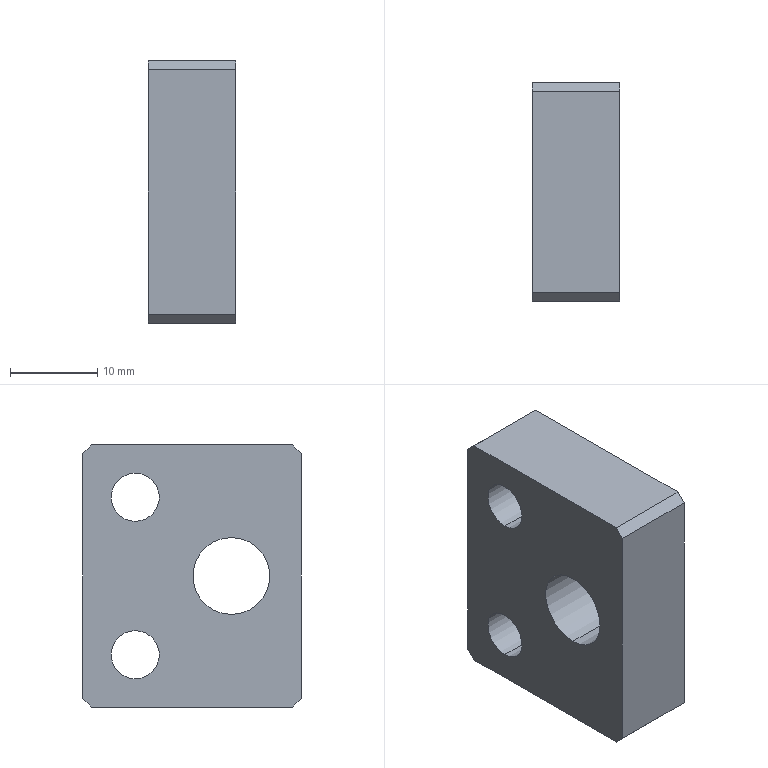Part | STEP file | PN_0052 | 1 solid | 22 faces | box 10 x 25 x 30 mm | volume 5805 mm3 | plane 12 | cylinder 10 | commonest cylinder face diameters 5.5 x4 10 x4 8.8 x2